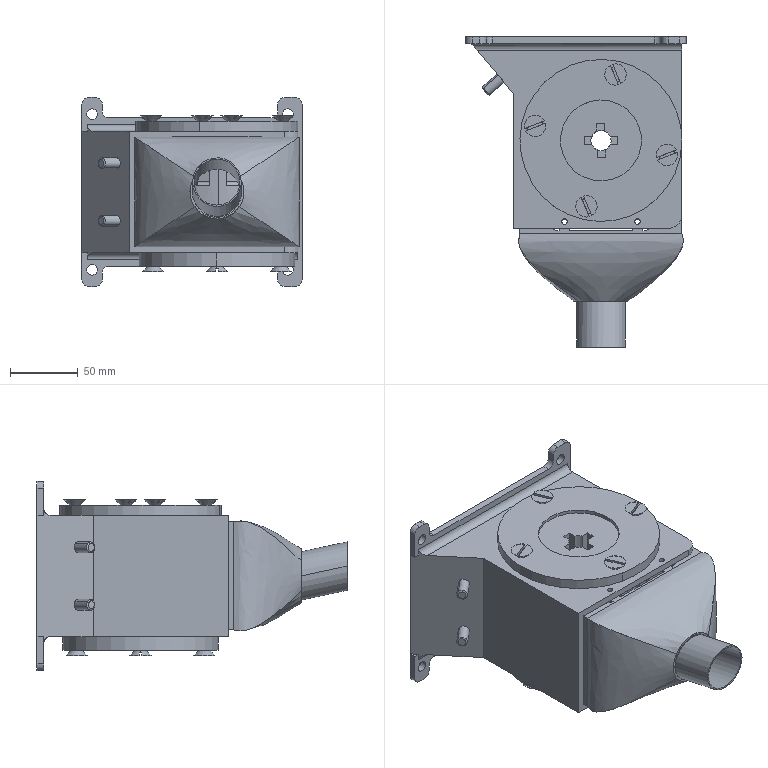Part | SolidWorks | features CompositeCurve 9, ReferencePattern 6, LocalCirPattern 2, MirrorCompFeat 1 | 18 solids | 1769 faces | box 163 x 229.711 x 140 mm | volume 1064629 mm3 | plane 1445 | cylinder 200 | cone 60 | spline 32 | torus 28 | sphere 4 | commonest cylinder face diameters 8 x40 6 x28 100 x21 10 x19 4 x16 6.918 x16